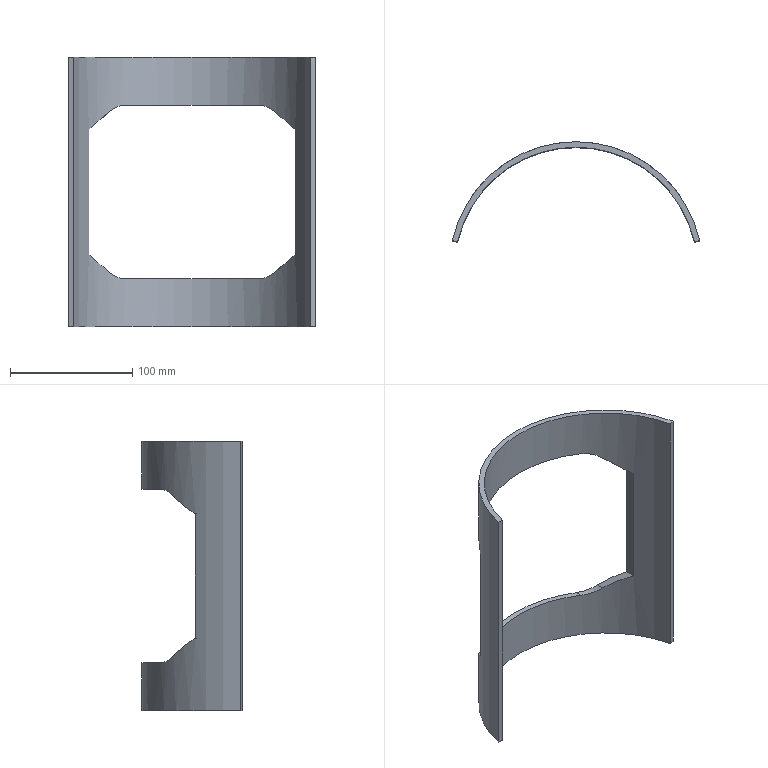Part | SolidWorks | features FlatPattern 1, ICE 1, SMBaseFlange 1, SheetMetal 1 | 1 solid | 18 faces | box 202.195 x 81.782 x 220 mm | volume 150063 mm3 | plane 12 | cylinder 6 | commonest cylinder face diameters 40 x4 198.3 x1 207.3 x1
STEP:
#1=CARTESIAN_POINT('',(101.098,22.861,0.));
#2=VERTEX_POINT('',#1);
#3=CARTESIAN_POINT('',(-101.098,22.861,0.));
#4=VERTEX_POINT('',#3);
#5=CARTESIAN_POINT('',(0.,0.,0.));
#6=DIRECTION('',(0.,0.,1.));
#7=DIRECTION('',(1.,0.,0.));
#8=AXIS2_PLACEMENT_3D('',#5,#6,#7);
#9=CIRCLE('',#8,103.65);
#10=EDGE_CURVE('',#2,#4,#9,.T.);
#11=ORIENTED_EDGE('',*,*,#10,.T.);
#12=CARTESIAN_POINT('',(-101.098,22.861,220.));
#13=VERTEX_POINT('',#12);
#14=CARTESIAN_POINT('',(-101.098,22.861,220.));
#15=DIRECTION('',(0.,0.,-1.));
#16=VECTOR('',#15,1000.);
#17=LINE('',#14,#16);
#18=EDGE_CURVE('',#13,#4,#17,.T.);
#19=ORIENTED_EDGE('',*,*,#18,.F.);
#20=CARTESIAN_POINT('',(101.098,22.861,220.));
#21=VERTEX_POINT('',#20);
#22=CARTESIAN_POINT('',(0.,0.,220.));
#23=DIRECTION('',(0.,0.,1.));
#24=DIRECTION('',(1.,0.,0.));
#25=AXIS2_PLACEMENT_3D('',#22,#23,#24);
#26=CIRCLE('',#25,103.65);
#27=EDGE_CURVE('',#21,#13,#26,.T.);
#28=ORIENTED_EDGE('',*,*,#27,.F.);
#29=CARTESIAN_POINT('',(101.098,22.861,220.));
#30=DIRECTION('',(0.,0.,-1.));
#31=VECTOR('',#30,1000.);
#32=LINE('',#29,#31);
#33=EDGE_CURVE('',#21,#2,#32,.T.);
#34=ORIENTED_EDGE('',*,*,#33,.T.);
#35=EDGE_LOOP('',(#11,#19,#28,#34));
#36=FACE_OUTER_BOUND('',#35,.T.);
#37=CARTESIAN_POINT('',(-68.475,77.811,175.025));
#38=VERTEX_POINT('',#37);
#39=CARTESIAN_POINT('',(-54.332,88.268,180.883));
#40=VERTEX_POINT('',#39);
#41=CARTESIAN_POINT('',(-68.475,77.811,175.025));
#42=CARTESIAN_POINT('',(-67.521,78.65,175.979));
#43=CARTESIAN_POINT('',(-66.504,79.514,176.806));
#44=CARTESIAN_POINT('',(-64.351,81.266,178.241));
#45=CARTESIAN_POINT('',(-63.215,82.155,178.85));
#46=CARTESIAN_POINT('',(-61.413,83.5,179.599));
#47=CARTESIAN_POINT('',(-60.796,83.951,179.821));
#48=CARTESIAN_POINT('',(-59.551,84.839,180.201));
#49=CARTESIAN_POINT('',(-58.919,85.279,180.361));
#50=CARTESIAN_POINT('',(-56.999,86.584,180.747));
#51=CARTESIAN_POINT('',(-55.685,87.436,180.883));
#52=CARTESIAN_POINT('',(-54.332,88.268,180.883));
#53=B_SPLINE_CURVE_WITH_KNOTS('',3,(#41,#42,#43,#44,#45,#46,#47,#48,#49,#50,#51,#52),.UNSPECIFIED.,.F.,.F.,(4,2,2,2,2,4),(0.,0.004688,0.009375,0.01172,0.01406,0.01875),.UNSPECIFIED.);
#54=EDGE_CURVE('',#38,#40,#53,.T.);
#55=ORIENTED_EDGE('',*,*,#54,.F.);
#56=CARTESIAN_POINT('',(-84.332,60.261,160.883));
#57=VERTEX_POINT('',#56);
#58=CARTESIAN_POINT('',(-84.332,60.261,160.883));
#59=CARTESIAN_POINT('',(-79.729,66.704,164.989));
#60=CARTESIAN_POINT('',(-74.419,72.579,169.724));
#61=CARTESIAN_POINT('',(-68.475,77.811,175.025));
#62=(BOUNDED_CURVE()B_SPLINE_CURVE(3,(#58,#59,#60,#61),.UNSPECIFIED.,.F.,.F.)B_SPLINE_CURVE_WITH_KNOTS((4,4),(0.6204,0.8491),.UNSPECIFIED.)CURVE()GEOMETRIC_REPRESENTATION_ITEM()RATIONAL_B_SPLINE_CURVE((1.,0.9956,0.9956,1.))REPRESENTATION_ITEM(''));
#63=EDGE_CURVE('',#57,#38,#62,.T.);
#64=ORIENTED_EDGE('',*,*,#63,.F.);
#65=CARTESIAN_POINT('',(-84.332,60.261,59.117));
#66=VERTEX_POINT('',#65);
#67=CARTESIAN_POINT('',(-84.332,60.261,220.));
#68=DIRECTION('',(0.,0.,1.));
#69=VECTOR('',#68,1000.);
#70=LINE('',#67,#69);
#71=EDGE_CURVE('',#66,#57,#70,.T.);
#72=ORIENTED_EDGE('',*,*,#71,.F.);
#73=CARTESIAN_POINT('',(-68.475,77.811,44.975));
#74=VERTEX_POINT('',#73);
#75=CARTESIAN_POINT('',(-68.475,77.811,44.975));
#76=CARTESIAN_POINT('',(-74.419,72.579,50.276));
#77=CARTESIAN_POINT('',(-79.729,66.704,55.011));
#78=CARTESIAN_POINT('',(-84.332,60.261,59.117));
#79=(BOUNDED_CURVE()B_SPLINE_CURVE(3,(#75,#76,#77,#78),.UNSPECIFIED.,.F.,.F.)B_SPLINE_CURVE_WITH_KNOTS((4,4),(2.292,2.521),.UNSPECIFIED.)CURVE()GEOMETRIC_REPRESENTATION_ITEM()RATIONAL_B_SPLINE_CURVE((1.,0.9956,0.9956,1.))REPRESENTATION_ITEM(''));
#80=EDGE_CURVE('',#74,#66,#79,.T.);
#81=ORIENTED_EDGE('',*,*,#80,.F.);
#82=CARTESIAN_POINT('',(-54.332,88.268,39.117));
#83=VERTEX_POINT('',#82);
#84=CARTESIAN_POINT('',(-54.332,88.268,39.117));
#85=CARTESIAN_POINT('',(-55.685,87.436,39.117));
#86=CARTESIAN_POINT('',(-56.997,86.585,39.253));
#87=CARTESIAN_POINT('',(-59.546,84.853,39.765));
#88=CARTESIAN_POINT('',(-60.784,83.97,40.141));
#89=CARTESIAN_POINT('',(-62.586,82.625,40.888));
#90=CARTESIAN_POINT('',(-63.178,82.173,41.167));
#91=CARTESIAN_POINT('',(-64.324,81.279,41.779));
#92=CARTESIAN_POINT('',(-64.88,80.835,42.112));
#93=CARTESIAN_POINT('',(-66.502,79.515,43.193));
#94=CARTESIAN_POINT('',(-67.521,78.65,44.021));
#95=CARTESIAN_POINT('',(-68.475,77.811,44.975));
#96=B_SPLINE_CURVE_WITH_KNOTS('',3,(#84,#85,#86,#87,#88,#89,#90,#91,#92,#93,#94,#95),.UNSPECIFIED.,.F.,.F.,(4,2,2,2,2,4),(0.,0.004687,0.009373,0.01172,0.01406,0.01875),.UNSPECIFIED.);
#97=EDGE_CURVE('',#83,#74,#96,.T.);
#98=ORIENTED_EDGE('',*,*,#97,.F.);
#99=CARTESIAN_POINT('',(54.332,88.268,39.117));
#100=VERTEX_POINT('',#99);
#101=CARTESIAN_POINT('',(0.,0.,39.117));
#102=DIRECTION('',(0.,0.,1.));
#103=DIRECTION('',(1.,0.,0.));
#104=AXIS2_PLACEMENT_3D('',#101,#102,#103);
#105=CIRCLE('',#104,103.65);
#106=EDGE_CURVE('',#100,#83,#105,.T.);
#107=ORIENTED_EDGE('',*,*,#106,.F.);
#108=CARTESIAN_POINT('',(68.475,77.811,44.975));
#109=VERTEX_POINT('',#108);
#110=CARTESIAN_POINT('',(68.475,77.811,44.975));
#111=CARTESIAN_POINT('',(67.521,78.65,44.021));
#112=CARTESIAN_POINT('',(66.504,79.514,43.194));
#113=CARTESIAN_POINT('',(64.351,81.266,41.759));
#114=CARTESIAN_POINT('',(63.215,82.155,41.15));
#115=CARTESIAN_POINT('',(61.413,83.5,40.401));
#116=CARTESIAN_POINT('',(60.796,83.951,40.179));
#117=CARTESIAN_POINT('',(59.551,84.839,39.799));
#118=CARTESIAN_POINT('',(58.919,85.279,39.639));
#119=CARTESIAN_POINT('',(56.999,86.584,39.253));
#120=CARTESIAN_POINT('',(55.685,87.436,39.117));
#121=CARTESIAN_POINT('',(54.332,88.268,39.117));
#122=B_SPLINE_CURVE_WITH_KNOTS('',3,(#110,#111,#112,#113,#114,#115,#116,#117,#118,#119,#120,#121),.UNSPECIFIED.,.F.,.F.,(4,2,2,2,2,4),(0.,0.004688,0.009375,0.01172,0.01406,0.01875),.UNSPECIFIED.);
#123=EDGE_CURVE('',#109,#100,#122,.T.);
#124=ORIENTED_EDGE('',*,*,#123,.F.);
#125=CARTESIAN_POINT('',(84.332,60.261,59.117));
#126=VERTEX_POINT('',#125);
#127=CARTESIAN_POINT('',(84.332,60.261,59.117));
#128=CARTESIAN_POINT('',(79.729,66.704,55.011));
#129=CARTESIAN_POINT('',(74.419,72.579,50.276));
#130=CARTESIAN_POINT('',(68.475,77.811,44.975));
#131=(BOUNDED_CURVE()B_SPLINE_CURVE(3,(#127,#128,#129,#130),.UNSPECIFIED.,.F.,.F.)B_SPLINE_CURVE_WITH_KNOTS((4,4),(3.762,3.991),.UNSPECIFIED.)CURVE()GEOMETRIC_REPRESENTATION_ITEM()RATIONAL_B_SPLINE_CURVE((1.,0.9956,0.9956,1.))REPRESENTATION_ITEM(''));
#132=EDGE_CURVE('',#126,#109,#131,.T.);
#133=ORIENTED_EDGE('',*,*,#132,.F.);
#134=CARTESIAN_POINT('',(84.332,60.261,160.883));
#135=VERTEX_POINT('',#134);
#136=CARTESIAN_POINT('',(84.332,60.261,220.));
#137=DIRECTION('',(0.,0.,-1.));
#138=VECTOR('',#137,1000.);
#139=LINE('',#136,#138);
#140=EDGE_CURVE('',#135,#126,#139,.T.);
#141=ORIENTED_EDGE('',*,*,#140,.F.);
#142=CARTESIAN_POINT('',(68.475,77.811,175.025));
#143=VERTEX_POINT('',#142);
#144=CARTESIAN_POINT('',(68.475,77.811,175.025));
#145=CARTESIAN_POINT('',(74.419,72.579,169.724));
#146=CARTESIAN_POINT('',(79.729,66.704,164.989));
#147=CARTESIAN_POINT('',(84.332,60.261,160.883));
#148=(BOUNDED_CURVE()B_SPLINE_CURVE(3,(#144,#145,#146,#147),.UNSPECIFIED.,.F.,.F.)B_SPLINE_CURVE_WITH_KNOTS((4,4),(5.434,5.663),.UNSPECIFIED.)CURVE()GEOMETRIC_REPRESENTATION_ITEM()RATIONAL_B_SPLINE_CURVE((1.,0.9956,0.9956,1.))REPRESENTATION_ITEM(''));
#149=EDGE_CURVE('',#143,#135,#148,.T.);
#150=ORIENTED_EDGE('',*,*,#149,.F.);
#151=CARTESIAN_POINT('',(54.332,88.268,180.883));
#152=VERTEX_POINT('',#151);
#153=CARTESIAN_POINT('',(54.332,88.268,180.883));
#154=CARTESIAN_POINT('',(55.685,87.436,180.883));
#155=CARTESIAN_POINT('',(56.997,86.585,180.747));
#156=CARTESIAN_POINT('',(59.546,84.853,180.235));
#157=CARTESIAN_POINT('',(60.784,83.97,179.859));
#158=CARTESIAN_POINT('',(62.586,82.625,179.112));
#159=CARTESIAN_POINT('',(63.178,82.173,178.833));
#160=CARTESIAN_POINT('',(64.324,81.279,178.221));
#161=CARTESIAN_POINT('',(64.88,80.835,177.888));
#162=CARTESIAN_POINT('',(66.502,79.515,176.807));
#163=CARTESIAN_POINT('',(67.521,78.65,175.979));
#164=CARTESIAN_POINT('',(68.475,77.811,175.025));
#165=B_SPLINE_CURVE_WITH_KNOTS('',3,(#153,#154,#155,#156,#157,#158,#159,#160,#161,#162,#163,#164),.UNSPECIFIED.,.F.,.F.,(4,2,2,2,2,4),(0.,0.004687,0.009373,0.01172,0.01406,0.01875),.UNSPECIFIED.);
#166=EDGE_CURVE('',#152,#143,#165,.T.);
#167=ORIENTED_EDGE('',*,*,#166,.F.);
#168=CARTESIAN_POINT('',(0.,0.,180.883));
#169=DIRECTION('',(0.,0.,-1.));
#170=DIRECTION('',(-1.,0.,0.));
#171=AXIS2_PLACEMENT_3D('',#168,#169,#170);
#172=CIRCLE('',#171,103.65);
#173=EDGE_CURVE('',#40,#152,#172,.T.);
#174=ORIENTED_EDGE('',*,*,#173,.F.);
#175=EDGE_LOOP('',(#55,#64,#72,#81,#98,#107,#124,#133,#141,#150,#167,#174));
#176=FACE_BOUND('',#175,.T.);
#177=CARTESIAN_POINT('',(0.,0.,220.));
#178=DIRECTION('',(0.,0.,-1.));
#179=DIRECTION('',(-1.,0.,0.));
#180=AXIS2_PLACEMENT_3D('',#177,#178,#179);
#181=CYLINDRICAL_SURFACE('',#180,103.65);
#182=ADVANCED_FACE('',(#36,#176),#181,.T.);
#183=CARTESIAN_POINT('',(96.708,21.868,0.));
#184=VERTEX_POINT('',#183);
#185=CARTESIAN_POINT('',(-96.708,21.868,0.));
#186=VERTEX_POINT('',#185);
#187=CARTESIAN_POINT('',(0.,0.,0.));
#188=DIRECTION('',(0.,0.,1.));
#189=DIRECTION('',(-1.,0.,0.));
#190=AXIS2_PLACEMENT_3D('',#187,#188,#189);
#191=CIRCLE('',#190,99.15);
#192=EDGE_CURVE('',#184,#186,#191,.T.);
#193=ORIENTED_EDGE('',*,*,#192,.F.);
#194=CARTESIAN_POINT('',(96.708,21.868,220.));
#195=VERTEX_POINT('',#194);
#196=CARTESIAN_POINT('',(96.708,21.868,220.));
#197=DIRECTION('',(0.,0.,-1.));
#198=VECTOR('',#197,1000.);
#199=LINE('',#196,#198);
#200=EDGE_CURVE('',#195,#184,#199,.T.);
#201=ORIENTED_EDGE('',*,*,#200,.F.);
#202=CARTESIAN_POINT('',(-96.708,21.868,220.));
#203=VERTEX_POINT('',#202);
#204=CARTESIAN_POINT('',(0.,0.,220.));
#205=DIRECTION('',(0.,0.,1.));
#206=DIRECTION('',(-1.,0.,0.));
#207=AXIS2_PLACEMENT_3D('',#204,#205,#206);
#208=CIRCLE('',#207,99.15);
#209=EDGE_CURVE('',#195,#203,#208,.T.);
#210=ORIENTED_EDGE('',*,*,#209,.T.);
#211=CARTESIAN_POINT('',(-96.708,21.868,220.));
#212=DIRECTION('',(0.,0.,-1.));
#213=VECTOR('',#212,1000.);
#214=LINE('',#211,#213);
#215=EDGE_CURVE('',#203,#186,#214,.T.);
#216=ORIENTED_EDGE('',*,*,#215,.T.);
#217=EDGE_LOOP('',(#193,#201,#210,#216));
#218=FACE_OUTER_BOUND('',#217,.T.);
#219=CARTESIAN_POINT('',(-84.332,52.142,160.883));
#220=VERTEX_POINT('',#219);
#221=CARTESIAN_POINT('',(-68.475,71.707,175.025));
#222=VERTEX_POINT('',#221);
#223=CARTESIAN_POINT('',(-84.332,52.142,160.883));
#224=CARTESIAN_POINT('',(-79.894,59.321,164.842));
#225=CARTESIAN_POINT('',(-74.579,65.878,169.581));
#226=CARTESIAN_POINT('',(-68.475,71.707,175.025));
#227=(BOUNDED_CURVE()B_SPLINE_CURVE(3,(#223,#224,#225,#226),.UNSPECIFIED.,.F.,.F.)B_SPLINE_CURVE_WITH_KNOTS((4,4),(0.5538,0.8085),.UNSPECIFIED.)CURVE()GEOMETRIC_REPRESENTATION_ITEM()RATIONAL_B_SPLINE_CURVE((1.,0.9946,0.9946,1.))REPRESENTATION_ITEM(''));
#228=EDGE_CURVE('',#220,#222,#227,.T.);
#229=ORIENTED_EDGE('',*,*,#228,.T.);
#230=CARTESIAN_POINT('',(-54.332,82.938,180.883));
#231=VERTEX_POINT('',#230);
#232=CARTESIAN_POINT('',(-68.475,71.707,175.025));
#233=CARTESIAN_POINT('',(-67.523,72.617,175.977));
#234=CARTESIAN_POINT('',(-66.508,73.549,176.803));
#235=CARTESIAN_POINT('',(-64.358,75.438,178.237));
#236=CARTESIAN_POINT('',(-63.222,76.394,178.846));
#237=CARTESIAN_POINT('',(-61.421,77.838,179.596));
#238=CARTESIAN_POINT('',(-60.806,78.32,179.818));
#239=CARTESIAN_POINT('',(-59.562,79.27,180.198));
#240=CARTESIAN_POINT('',(-58.931,79.74,180.358));
#241=CARTESIAN_POINT('',(-57.009,81.137,180.746));
#242=CARTESIAN_POINT('',(-55.691,82.048,180.883));
#243=CARTESIAN_POINT('',(-54.332,82.938,180.883));
#244=B_SPLINE_CURVE_WITH_KNOTS('',3,(#232,#233,#234,#235,#236,#237,#238,#239,#240,#241,#242,#243),.UNSPECIFIED.,.F.,.F.,(4,2,2,2,2,4),(0.,0.004802,0.009603,0.012,0.0144,0.01921),.UNSPECIFIED.);
#245=EDGE_CURVE('',#222,#231,#244,.T.);
#246=ORIENTED_EDGE('',*,*,#245,.T.);
#247=CARTESIAN_POINT('',(54.332,82.938,180.883));
#248=VERTEX_POINT('',#247);
#249=CARTESIAN_POINT('',(0.,0.,180.883));
#250=DIRECTION('',(0.,0.,-1.));
#251=DIRECTION('',(-1.,0.,0.));
#252=AXIS2_PLACEMENT_3D('',#249,#250,#251);
#253=CIRCLE('',#252,99.15);
#254=EDGE_CURVE('',#231,#248,#253,.T.);
#255=ORIENTED_EDGE('',*,*,#254,.T.);
#256=CARTESIAN_POINT('',(68.475,71.707,175.025));
#257=VERTEX_POINT('',#256);
#258=CARTESIAN_POINT('',(54.332,82.938,180.883));
#259=CARTESIAN_POINT('',(55.692,82.047,180.883));
#260=CARTESIAN_POINT('',(57.008,81.138,180.746));
#261=CARTESIAN_POINT('',(59.563,79.281,180.231));
#262=CARTESIAN_POINT('',(60.801,78.335,179.853));
#263=CARTESIAN_POINT('',(62.603,76.891,179.105));
#264=CARTESIAN_POINT('',(63.193,76.407,178.825));
#265=CARTESIAN_POINT('',(64.335,75.448,178.215));
#266=CARTESIAN_POINT('',(64.889,74.971,177.882));
#267=CARTESIAN_POINT('',(66.507,73.55,176.804));
#268=CARTESIAN_POINT('',(67.523,72.616,175.977));
#269=CARTESIAN_POINT('',(68.475,71.707,175.025));
#270=B_SPLINE_CURVE_WITH_KNOTS('',3,(#258,#259,#260,#261,#262,#263,#264,#265,#266,#267,#268,#269),.UNSPECIFIED.,.F.,.F.,(4,2,2,2,2,4),(0.,0.004799,0.009599,0.012,0.0144,0.0192),.UNSPECIFIED.);
#271=EDGE_CURVE('',#248,#257,#270,.T.);
#272=ORIENTED_EDGE('',*,*,#271,.T.);
#273=CARTESIAN_POINT('',(84.332,52.142,160.883));
#274=VERTEX_POINT('',#273);
#275=CARTESIAN_POINT('',(68.475,71.707,175.025));
#276=CARTESIAN_POINT('',(74.579,65.878,169.581));
#277=CARTESIAN_POINT('',(79.894,59.321,164.842));
#278=CARTESIAN_POINT('',(84.332,52.142,160.883));
#279=(BOUNDED_CURVE()B_SPLINE_CURVE(3,(#275,#276,#277,#278),.UNSPECIFIED.,.F.,.F.)B_SPLINE_CURVE_WITH_KNOTS((4,4),(5.475,5.729),.UNSPECIFIED.)CURVE()GEOMETRIC_REPRESENTATION_ITEM()RATIONAL_B_SPLINE_CURVE((1.,0.9946,0.9946,1.))REPRESENTATION_ITEM(''));
#280=EDGE_CURVE('',#257,#274,#279,.T.);
#281=ORIENTED_EDGE('',*,*,#280,.T.);
#282=CARTESIAN_POINT('',(84.332,52.142,59.117));
#283=VERTEX_POINT('',#282);
#284=CARTESIAN_POINT('',(84.332,52.142,220.));
#285=DIRECTION('',(0.,0.,-1.));
#286=VECTOR('',#285,1000.);
#287=LINE('',#284,#286);
#288=EDGE_CURVE('',#274,#283,#287,.T.);
#289=ORIENTED_EDGE('',*,*,#288,.T.);
#290=CARTESIAN_POINT('',(68.475,71.707,44.975));
#291=VERTEX_POINT('',#290);
#292=CARTESIAN_POINT('',(84.332,52.142,59.117));
#293=CARTESIAN_POINT('',(79.894,59.321,55.158));
#294=CARTESIAN_POINT('',(74.579,65.878,50.419));
#295=CARTESIAN_POINT('',(68.475,71.707,44.975));
#296=(BOUNDED_CURVE()B_SPLINE_CURVE(3,(#292,#293,#294,#295),.UNSPECIFIED.,.F.,.F.)B_SPLINE_CURVE_WITH_KNOTS((4,4),(3.695,3.95),.UNSPECIFIED.)CURVE()GEOMETRIC_REPRESENTATION_ITEM()RATIONAL_B_SPLINE_CURVE((1.,0.9946,0.9946,1.))REPRESENTATION_ITEM(''));
#297=EDGE_CURVE('',#283,#291,#296,.T.);
#298=ORIENTED_EDGE('',*,*,#297,.T.);
#299=CARTESIAN_POINT('',(54.332,82.938,39.117));
#300=VERTEX_POINT('',#299);
#301=CARTESIAN_POINT('',(68.475,71.707,44.975));
#302=CARTESIAN_POINT('',(67.523,72.617,44.023));
#303=CARTESIAN_POINT('',(66.508,73.549,43.197));
#304=CARTESIAN_POINT('',(64.358,75.438,41.763));
#305=CARTESIAN_POINT('',(63.222,76.394,41.154));
#306=CARTESIAN_POINT('',(61.421,77.838,40.404));
#307=CARTESIAN_POINT('',(60.806,78.32,40.182));
#308=CARTESIAN_POINT('',(59.562,79.27,39.802));
#309=CARTESIAN_POINT('',(58.931,79.74,39.642));
#310=CARTESIAN_POINT('',(57.009,81.137,39.254));
#311=CARTESIAN_POINT('',(55.691,82.048,39.117));
#312=CARTESIAN_POINT('',(54.332,82.938,39.117));
#313=B_SPLINE_CURVE_WITH_KNOTS('',3,(#301,#302,#303,#304,#305,#306,#307,#308,#309,#310,#311,#312),.UNSPECIFIED.,.F.,.F.,(4,2,2,2,2,4),(0.,0.004802,0.009603,0.012,0.0144,0.01921),.UNSPECIFIED.);
#314=EDGE_CURVE('',#291,#300,#313,.T.);
#315=ORIENTED_EDGE('',*,*,#314,.T.);
#316=CARTESIAN_POINT('',(-54.332,82.938,39.117));
#317=VERTEX_POINT('',#316);
#318=CARTESIAN_POINT('',(0.,0.,39.117));
#319=DIRECTION('',(0.,0.,1.));
#320=DIRECTION('',(1.,0.,0.));
#321=AXIS2_PLACEMENT_3D('',#318,#319,#320);
#322=CIRCLE('',#321,99.15);
#323=EDGE_CURVE('',#300,#317,#322,.T.);
#324=ORIENTED_EDGE('',*,*,#323,.T.);
#325=CARTESIAN_POINT('',(-68.475,71.707,44.975));
#326=VERTEX_POINT('',#325);
#327=CARTESIAN_POINT('',(-54.332,82.938,39.117));
#328=CARTESIAN_POINT('',(-55.692,82.047,39.117));
#329=CARTESIAN_POINT('',(-57.008,81.138,39.254));
#330=CARTESIAN_POINT('',(-59.563,79.281,39.769));
#331=CARTESIAN_POINT('',(-60.801,78.335,40.147));
#332=CARTESIAN_POINT('',(-62.603,76.891,40.895));
#333=CARTESIAN_POINT('',(-63.193,76.407,41.175));
#334=CARTESIAN_POINT('',(-64.335,75.448,41.785));
#335=CARTESIAN_POINT('',(-64.889,74.971,42.118));
#336=CARTESIAN_POINT('',(-66.507,73.55,43.196));
#337=CARTESIAN_POINT('',(-67.523,72.616,44.023));
#338=CARTESIAN_POINT('',(-68.475,71.707,44.975));
#339=B_SPLINE_CURVE_WITH_KNOTS('',3,(#327,#328,#329,#330,#331,#332,#333,#334,#335,#336,#337,#338),.UNSPECIFIED.,.F.,.F.,(4,2,2,2,2,4),(0.,0.004799,0.009599,0.012,0.0144,0.0192),.UNSPECIFIED.);
#340=EDGE_CURVE('',#317,#326,#339,.T.);
#341=ORIENTED_EDGE('',*,*,#340,.T.);
#342=CARTESIAN_POINT('',(-84.332,52.142,59.117));
#343=VERTEX_POINT('',#342);
#344=CARTESIAN_POINT('',(-68.475,71.707,44.975));
#345=CARTESIAN_POINT('',(-74.579,65.878,50.419));
#346=CARTESIAN_POINT('',(-79.894,59.321,55.158));
#347=CARTESIAN_POINT('',(-84.332,52.142,59.117));
#348=(BOUNDED_CURVE()B_SPLINE_CURVE(3,(#344,#345,#346,#347),.UNSPECIFIED.,.F.,.F.)B_SPLINE_CURVE_WITH_KNOTS((4,4),(2.333,2.588),.UNSPECIFIED.)CURVE()GEOMETRIC_REPRESENTATION_ITEM()RATIONAL_B_SPLINE_CURVE((1.,0.9946,0.9946,1.))REPRESENTATION_ITEM(''));
#349=EDGE_CURVE('',#326,#343,#348,.T.);
#350=ORIENTED_EDGE('',*,*,#349,.T.);
#351=CARTESIAN_POINT('',(-84.332,52.142,220.));
#352=DIRECTION('',(0.,0.,1.));
#353=VECTOR('',#352,1000.);
#354=LINE('',#351,#353);
#355=EDGE_CURVE('',#343,#220,#354,.T.);
#356=ORIENTED_EDGE('',*,*,#355,.T.);
#357=EDGE_LOOP('',(#229,#246,#255,#272,#281,#289,#298,#315,#324,#341,#350,#356));
#358=FACE_BOUND('',#357,.T.);
#359=CARTESIAN_POINT('',(0.,0.,220.));
#360=DIRECTION('',(0.,0.,-1.));
#361=DIRECTION('',(-1.,0.,0.));
#362=AXIS2_PLACEMENT_3D('',#359,#360,#361);
#363=CYLINDRICAL_SURFACE('',#362,99.15);
#364=ADVANCED_FACE('',(#218,#358),#363,.F.);
#365=CARTESIAN_POINT('',(-96.708,21.868,0.));
#366=DIRECTION('',(-0.9754,0.2206,0.));
#367=VECTOR('',#366,1000.);
#368=LINE('',#365,#367);
#369=EDGE_CURVE('',#186,#4,#368,.T.);
#370=ORIENTED_EDGE('',*,*,#369,.F.);
#371=ORIENTED_EDGE('',*,*,#215,.F.);
#372=CARTESIAN_POINT('',(-96.708,21.868,220.));
#373=DIRECTION('',(-0.9754,0.2206,0.));
#374=VECTOR('',#373,1000.);
#375=LINE('',#372,#374);
#376=EDGE_CURVE('',#203,#13,#375,.T.);
#377=ORIENTED_EDGE('',*,*,#376,.T.);
#378=ORIENTED_EDGE('',*,*,#18,.T.);
#379=EDGE_LOOP('',(#370,#371,#377,#378));
#380=FACE_OUTER_BOUND('',#379,.T.);
#381=CARTESIAN_POINT('',(-96.708,21.868,220.));
#382=DIRECTION('',(-0.2206,-0.9754,0.));
#383=DIRECTION('',(0.9754,-0.2206,0.));
#384=AXIS2_PLACEMENT_3D('',#381,#382,#383);
#385=PLANE('',#384);
#386=ADVANCED_FACE('',(#380),#385,.T.);
#387=CARTESIAN_POINT('',(101.098,22.861,0.));
#388=DIRECTION('',(-0.9754,-0.2206,0.));
#389=VECTOR('',#388,1000.);
#390=LINE('',#387,#389);
#391=EDGE_CURVE('',#2,#184,#390,.T.);
#392=ORIENTED_EDGE('',*,*,#391,.F.);
#393=ORIENTED_EDGE('',*,*,#33,.F.);
#394=CARTESIAN_POINT('',(101.098,22.861,220.));
#395=DIRECTION('',(-0.9754,-0.2206,0.));
#396=VECTOR('',#395,1000.);
#397=LINE('',#394,#396);
#398=EDGE_CURVE('',#21,#195,#397,.T.);
#399=ORIENTED_EDGE('',*,*,#398,.T.);
#400=ORIENTED_EDGE('',*,*,#200,.T.);
#401=EDGE_LOOP('',(#392,#393,#399,#400));
#402=FACE_OUTER_BOUND('',#401,.T.);
#403=CARTESIAN_POINT('',(101.098,22.861,220.));
#404=DIRECTION('',(0.2206,-0.9754,0.));
#405=DIRECTION('',(0.9754,0.2206,0.));
#406=AXIS2_PLACEMENT_3D('',#403,#404,#405);
#407=PLANE('',#406);
#408=ADVANCED_FACE('',(#402),#407,.T.);
#409=ORIENTED_EDGE('',*,*,#27,.T.);
#410=ORIENTED_EDGE('',*,*,#376,.F.);
#411=ORIENTED_EDGE('',*,*,#209,.F.);
#412=ORIENTED_EDGE('',*,*,#398,.F.);
#413=EDGE_LOOP('',(#409,#410,#411,#412));
#414=FACE_OUTER_BOUND('',#413,.T.);
#415=CARTESIAN_POINT('',(0.,0.,220.));
#416=DIRECTION('',(0.,0.,1.));
#417=DIRECTION('',(-1.,0.,0.));
#418=AXIS2_PLACEMENT_3D('',#415,#416,#417);
#419=PLANE('',#418);
#420=ADVANCED_FACE('',(#414),#419,.T.);
#421=ORIENTED_EDGE('',*,*,#10,.F.);
#422=ORIENTED_EDGE('',*,*,#391,.T.);
#423=ORIENTED_EDGE('',*,*,#192,.T.);
#424=ORIENTED_EDGE('',*,*,#369,.T.);
#425=EDGE_LOOP('',(#421,#422,#423,#424));
#426=FACE_OUTER_BOUND('',#425,.T.);
#427=CARTESIAN_POINT('',(0.,0.,0.));
#428=DIRECTION('',(0.,0.,1.));
#429=DIRECTION('',(-1.,0.,0.));
#430=AXIS2_PLACEMENT_3D('',#427,#428,#429);
#431=PLANE('',#430);
#432=ADVANCED_FACE('',(#426),#431,.F.);
#433=ORIENTED_EDGE('',*,*,#54,.T.);
#434=CARTESIAN_POINT('',(-54.332,141.,180.883));
#435=DIRECTION('',(0.,-1.,0.));
#436=VECTOR('',#435,1000.);
#437=LINE('',#434,#436);
#438=EDGE_CURVE('',#40,#231,#437,.T.);
#439=ORIENTED_EDGE('',*,*,#438,.T.);
#440=ORIENTED_EDGE('',*,*,#245,.F.);
#441=CARTESIAN_POINT('',(-68.475,141.,175.025));
#442=DIRECTION('',(0.,-1.,0.));
#443=VECTOR('',#442,1000.);
#444=LINE('',#441,#443);
#445=EDGE_CURVE('',#38,#222,#444,.T.);
#446=ORIENTED_EDGE('',*,*,#445,.F.);
#447=EDGE_LOOP('',(#433,#439,#440,#446));
#448=FACE_OUTER_BOUND('',#447,.T.);
#449=CARTESIAN_POINT('',(-54.332,141.,160.883));
#450=DIRECTION('',(0.,-1.,0.));
#451=DIRECTION('',(0.,0.,-1.));
#452=AXIS2_PLACEMENT_3D('',#449,#450,#451);
#453=CYLINDRICAL_SURFACE('',#452,20.);
#454=ADVANCED_FACE('',(#448),#453,.F.);
#455=ORIENTED_EDGE('',*,*,#173,.T.);
#456=CARTESIAN_POINT('',(54.332,141.,180.883));
#457=DIRECTION('',(0.,-1.,0.));
#458=VECTOR('',#457,1000.);
#459=LINE('',#456,#458);
#460=EDGE_CURVE('',#152,#248,#459,.T.);
#461=ORIENTED_EDGE('',*,*,#460,.T.);
#462=ORIENTED_EDGE('',*,*,#254,.F.);
#463=ORIENTED_EDGE('',*,*,#438,.F.);
#464=EDGE_LOOP('',(#455,#461,#462,#463));
#465=FACE_OUTER_BOUND('',#464,.T.);
#466=CARTESIAN_POINT('',(-54.332,141.,180.883));
#467=DIRECTION('',(0.,0.,-1.));
#468=DIRECTION('',(-1.,0.,0.));
#469=AXIS2_PLACEMENT_3D('',#466,#467,#468);
#470=PLANE('',#469);
#471=ADVANCED_FACE('',(#465),#470,.T.);
#472=ORIENTED_EDGE('',*,*,#166,.T.);
#473=CARTESIAN_POINT('',(68.475,141.,175.025));
#474=DIRECTION('',(0.,-1.,0.));
#475=VECTOR('',#474,1000.);
#476=LINE('',#473,#475);
#477=EDGE_CURVE('',#143,#257,#476,.T.);
#478=ORIENTED_EDGE('',*,*,#477,.T.);
#479=ORIENTED_EDGE('',*,*,#271,.F.);
#480=ORIENTED_EDGE('',*,*,#460,.F.);
#481=EDGE_LOOP('',(#472,#478,#479,#480));
#482=FACE_OUTER_BOUND('',#481,.T.);
#483=CARTESIAN_POINT('',(54.332,141.,160.883));
#484=DIRECTION('',(0.,-1.,0.));
#485=DIRECTION('',(0.,0.,-1.));
#486=AXIS2_PLACEMENT_3D('',#483,#484,#485);
#487=CYLINDRICAL_SURFACE('',#486,20.);
#488=ADVANCED_FACE('',(#482),#487,.F.);
#489=ORIENTED_EDGE('',*,*,#149,.T.);
#490=CARTESIAN_POINT('',(84.332,141.,160.883));
#491=DIRECTION('',(0.,-1.,0.));
#492=VECTOR('',#491,1000.);
#493=LINE('',#490,#492);
#494=EDGE_CURVE('',#135,#274,#493,.T.);
#495=ORIENTED_EDGE('',*,*,#494,.T.);
#496=ORIENTED_EDGE('',*,*,#280,.F.);
#497=ORIENTED_EDGE('',*,*,#477,.F.);
#498=EDGE_LOOP('',(#489,#495,#496,#497));
#499=FACE_OUTER_BOUND('',#498,.T.);
#500=CARTESIAN_POINT('',(84.332,141.,160.883));
#501=DIRECTION('',(-0.6656,0.,-0.7463));
#502=DIRECTION('',(-0.7463,0.,0.6656));
#503=AXIS2_PLACEMENT_3D('',#500,#501,#502);
#504=PLANE('',#503);
#505=ADVANCED_FACE('',(#499),#504,.T.);
#506=ORIENTED_EDGE('',*,*,#140,.T.);
#507=CARTESIAN_POINT('',(84.332,141.,59.117));
#508=DIRECTION('',(0.,-1.,0.));
#509=VECTOR('',#508,1000.);
#510=LINE('',#507,#509);
#511=EDGE_CURVE('',#126,#283,#510,.T.);
#512=ORIENTED_EDGE('',*,*,#511,.T.);
#513=ORIENTED_EDGE('',*,*,#288,.F.);
#514=ORIENTED_EDGE('',*,*,#494,.F.);
#515=EDGE_LOOP('',(#506,#512,#513,#514));
#516=FACE_OUTER_BOUND('',#515,.T.);
#517=CARTESIAN_POINT('',(84.332,141.,59.117));
#518=DIRECTION('',(-1.,0.,0.));
#519=DIRECTION('',(0.,0.,1.));
#520=AXIS2_PLACEMENT_3D('',#517,#518,#519);
#521=PLANE('',#520);
#522=ADVANCED_FACE('',(#516),#521,.T.);
#523=ORIENTED_EDGE('',*,*,#132,.T.);
#524=CARTESIAN_POINT('',(68.475,141.,44.975));
#525=DIRECTION('',(0.,-1.,0.));
#526=VECTOR('',#525,1000.);
#527=LINE('',#524,#526);
#528=EDGE_CURVE('',#109,#291,#527,.T.);
#529=ORIENTED_EDGE('',*,*,#528,.T.);
#530=ORIENTED_EDGE('',*,*,#297,.F.);
#531=ORIENTED_EDGE('',*,*,#511,.F.);
#532=EDGE_LOOP('',(#523,#529,#530,#531));
#533=FACE_OUTER_BOUND('',#532,.T.);
#534=CARTESIAN_POINT('',(84.332,141.,59.117));
#535=DIRECTION('',(-0.6656,0.,0.7463));
#536=DIRECTION('',(0.7463,0.,0.6656));
#537=AXIS2_PLACEMENT_3D('',#534,#535,#536);
#538=PLANE('',#537);
#539=ADVANCED_FACE('',(#533),#538,.T.);
#540=ORIENTED_EDGE('',*,*,#123,.T.);
#541=CARTESIAN_POINT('',(54.332,141.,39.117));
#542=DIRECTION('',(0.,-1.,0.));
#543=VECTOR('',#542,1000.);
#544=LINE('',#541,#543);
#545=EDGE_CURVE('',#100,#300,#544,.T.);
#546=ORIENTED_EDGE('',*,*,#545,.T.);
#547=ORIENTED_EDGE('',*,*,#314,.F.);
#548=ORIENTED_EDGE('',*,*,#528,.F.);
#549=EDGE_LOOP('',(#540,#546,#547,#548));
#550=FACE_OUTER_BOUND('',#549,.T.);
#551=CARTESIAN_POINT('',(54.332,141.,59.117));
#552=DIRECTION('',(0.,-1.,0.));
#553=DIRECTION('',(0.,0.,-1.));
#554=AXIS2_PLACEMENT_3D('',#551,#552,#553);
#555=CYLINDRICAL_SURFACE('',#554,20.);
#556=ADVANCED_FACE('',(#550),#555,.F.);
#557=ORIENTED_EDGE('',*,*,#106,.T.);
#558=CARTESIAN_POINT('',(-54.332,141.,39.117));
#559=DIRECTION('',(0.,-1.,0.));
#560=VECTOR('',#559,1000.);
#561=LINE('',#558,#560);
#562=EDGE_CURVE('',#83,#317,#561,.T.);
#563=ORIENTED_EDGE('',*,*,#562,.T.);
#564=ORIENTED_EDGE('',*,*,#323,.F.);
#565=ORIENTED_EDGE('',*,*,#545,.F.);
#566=EDGE_LOOP('',(#557,#563,#564,#565));
#567=FACE_OUTER_BOUND('',#566,.T.);
#568=CARTESIAN_POINT('',(-54.332,141.,39.117));
#569=DIRECTION('',(0.,0.,1.));
#570=DIRECTION('',(1.,0.,0.));
#571=AXIS2_PLACEMENT_3D('',#568,#569,#570);
#572=PLANE('',#571);
#573=ADVANCED_FACE('',(#567),#572,.T.);
#574=ORIENTED_EDGE('',*,*,#97,.T.);
#575=CARTESIAN_POINT('',(-68.475,141.,44.975));
#576=DIRECTION('',(0.,-1.,0.));
#577=VECTOR('',#576,1000.);
#578=LINE('',#575,#577);
#579=EDGE_CURVE('',#74,#326,#578,.T.);
#580=ORIENTED_EDGE('',*,*,#579,.T.);
#581=ORIENTED_EDGE('',*,*,#340,.F.);
#582=ORIENTED_EDGE('',*,*,#562,.F.);
#583=EDGE_LOOP('',(#574,#580,#581,#582));
#584=FACE_OUTER_BOUND('',#583,.T.);
#585=CARTESIAN_POINT('',(-54.332,141.,59.117));
#586=DIRECTION('',(0.,-1.,0.));
#587=DIRECTION('',(0.,0.,-1.));
#588=AXIS2_PLACEMENT_3D('',#585,#586,#587);
#589=CYLINDRICAL_SURFACE('',#588,20.);
#590=ADVANCED_FACE('',(#584),#589,.F.);
#591=ORIENTED_EDGE('',*,*,#80,.T.);
#592=CARTESIAN_POINT('',(-84.332,141.,59.117));
#593=DIRECTION('',(0.,-1.,0.));
#594=VECTOR('',#593,1000.);
#595=LINE('',#592,#594);
#596=EDGE_CURVE('',#66,#343,#595,.T.);
#597=ORIENTED_EDGE('',*,*,#596,.T.);
#598=ORIENTED_EDGE('',*,*,#349,.F.);
#599=ORIENTED_EDGE('',*,*,#579,.F.);
#600=EDGE_LOOP('',(#591,#597,#598,#599));
#601=FACE_OUTER_BOUND('',#600,.T.);
#602=CARTESIAN_POINT('',(-84.332,141.,59.117));
#603=DIRECTION('',(0.6656,0.,0.7463));
#604=DIRECTION('',(0.7463,0.,-0.6656));
#605=AXIS2_PLACEMENT_3D('',#602,#603,#604);
#606=PLANE('',#605);
#607=ADVANCED_FACE('',(#601),#606,.T.);
#608=ORIENTED_EDGE('',*,*,#71,.T.);
#609=CARTESIAN_POINT('',(-84.332,141.,160.883));
#610=DIRECTION('',(0.,-1.,0.));
#611=VECTOR('',#610,1000.);
#612=LINE('',#609,#611);
#613=EDGE_CURVE('',#57,#220,#612,.T.);
#614=ORIENTED_EDGE('',*,*,#613,.T.);
#615=ORIENTED_EDGE('',*,*,#355,.F.);
#616=ORIENTED_EDGE('',*,*,#596,.F.);
#617=EDGE_LOOP('',(#608,#614,#615,#616));
#618=FACE_OUTER_BOUND('',#617,.T.);
#619=CARTESIAN_POINT('',(-84.332,141.,59.117));
#620=DIRECTION('',(1.,0.,0.));
#621=DIRECTION('',(0.,0.,-1.));
#622=AXIS2_PLACEMENT_3D('',#619,#620,#621);
#623=PLANE('',#622);
#624=ADVANCED_FACE('',(#618),#623,.T.);
#625=ORIENTED_EDGE('',*,*,#63,.T.);
#626=ORIENTED_EDGE('',*,*,#445,.T.);
#627=ORIENTED_EDGE('',*,*,#228,.F.);
#628=ORIENTED_EDGE('',*,*,#613,.F.);
#629=EDGE_LOOP('',(#625,#626,#627,#628));
#630=FACE_OUTER_BOUND('',#629,.T.);
#631=CARTESIAN_POINT('',(-84.332,141.,160.883));
#632=DIRECTION('',(0.6656,0.,-0.7463));
#633=DIRECTION('',(-0.7463,0.,-0.6656));
#634=AXIS2_PLACEMENT_3D('',#631,#632,#633);
#635=PLANE('',#634);
#636=ADVANCED_FACE('',(#630),#635,.T.);
#637=CLOSED_SHELL('',(#182,#364,#386,#408,#420,#432,#454,#471,#488,#505,#522,#539,#556,#573,#590,#607,#624,#636));
#638=MANIFOLD_SOLID_BREP('',#637);
#639=CARTESIAN_POINT('',(0.,0.,0.));
#640=DIRECTION('',(0.,0.,1.));
#641=DIRECTION('',(1.,0.,0.));
#642=AXIS2_PLACEMENT_3D('',#639,#640,#641);
#643=(LENGTH_UNIT()NAMED_UNIT(*)SI_UNIT(.MILLI.,.METRE.));
#644=UNCERTAINTY_MEASURE_WITH_UNIT(LENGTH_MEASURE(0.00001),#643,'','');
#645=(NAMED_UNIT(*)PLANE_ANGLE_UNIT()SI_UNIT($,.RADIAN.));
#646=(NAMED_UNIT(*)SI_UNIT($,.STERADIAN.)SOLID_ANGLE_UNIT());
#647=(GEOMETRIC_REPRESENTATION_CONTEXT(3)GLOBAL_UNCERTAINTY_ASSIGNED_CONTEXT((#644))GLOBAL_UNIT_ASSIGNED_CONTEXT((#643,#645,#646))REPRESENTATION_CONTEXT('',''));
#648=ADVANCED_BREP_SHAPE_REPRESENTATION('',(#638,#642),#647);